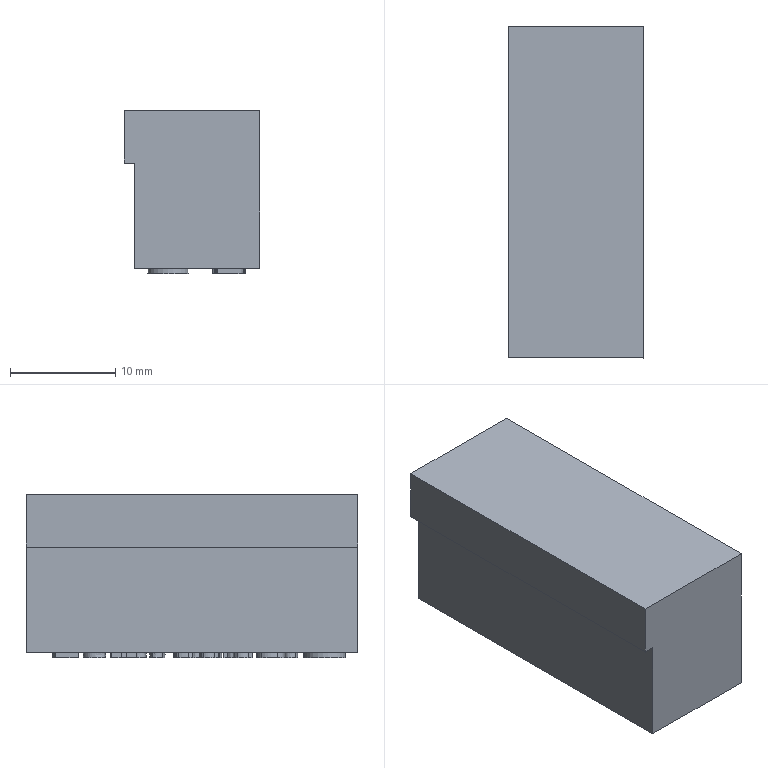Part | STEP file | gslz 2016.10.28-10_id3154_x_t | 1 solid | 316 faces | box 12.88 x 31.5 x 15.5 mm | volume 5788 mm3 | plane 148 | other 142 | cylinder 26 | commonest cylinder face diameters 2.659 x5 0.649 x1 1.171 x1 1.215 x1 1.37 x1 1.755 x1